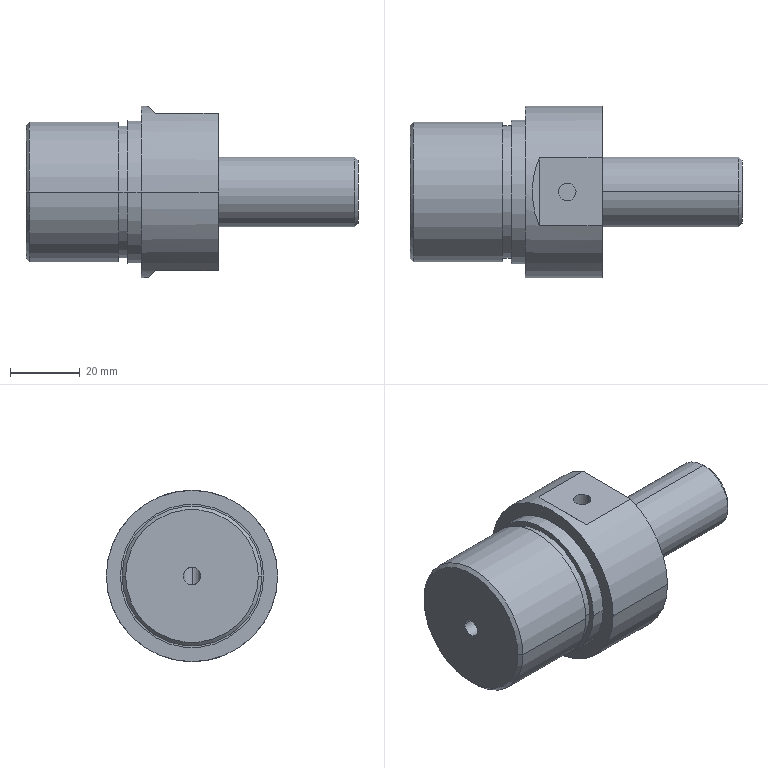Part | SolidWorks | features ICE 4, Chamfer 2, BaseBody 1, MoveFace 1 | 1 solid | 29 faces | box 95 x 49 x 49 mm | volume 93064 mm3 | cylinder 14 | plane 11 | cone 4 | commonest cylinder face diameters 5 x4 20 x2 38 x2 40 x2 41 x2 49 x2
STEP:
#1=CARTESIAN_POINT('',(82.,0.,-9.));
#2=VERTEX_POINT('',#1);
#3=CARTESIAN_POINT('',(82.,0.,9.));
#4=VERTEX_POINT('',#3);
#5=CARTESIAN_POINT('',(82.,0.,0.));
#6=DIRECTION('',(1.,0.,0.));
#7=DIRECTION('',(0.,0.,-1.));
#8=AXIS2_PLACEMENT_3D('',#5,#6,#7);
#9=CIRCLE('',#8,9.);
#10=EDGE_CURVE('',#2,#4,#9,.T.);
#11=ORIENTED_EDGE('',*,*,#10,.F.);
#12=CARTESIAN_POINT('',(81.,0.,-10.));
#13=VERTEX_POINT('',#12);
#14=CARTESIAN_POINT('',(81.,0.,-10.));
#15=DIRECTION('',(-0.7071,0.,-0.7071));
#16=VECTOR('',#15,1000.);
#17=LINE('',#14,#16);
#18=EDGE_CURVE('',#2,#13,#17,.T.);
#19=ORIENTED_EDGE('',*,*,#18,.T.);
#20=CARTESIAN_POINT('',(81.,0.,10.));
#21=VERTEX_POINT('',#20);
#22=CARTESIAN_POINT('',(81.,0.,0.));
#23=DIRECTION('',(-1.,0.,0.));
#24=DIRECTION('',(0.,0.,-1.));
#25=AXIS2_PLACEMENT_3D('',#22,#23,#24);
#26=CIRCLE('',#25,10.);
#27=EDGE_CURVE('',#21,#13,#26,.T.);
#28=ORIENTED_EDGE('',*,*,#27,.F.);
#29=CARTESIAN_POINT('',(81.,0.,10.));
#30=DIRECTION('',(-0.7071,0.,0.7071));
#31=VECTOR('',#30,1000.);
#32=LINE('',#29,#31);
#33=EDGE_CURVE('',#4,#21,#32,.T.);
#34=ORIENTED_EDGE('',*,*,#33,.F.);
#35=EDGE_LOOP('',(#11,#19,#28,#34));
#36=FACE_OUTER_BOUND('',#35,.T.);
#37=CARTESIAN_POINT('',(81.,0.,0.));
#38=DIRECTION('',(-1.,0.,0.));
#39=DIRECTION('',(0.,0.,1.));
#40=AXIS2_PLACEMENT_3D('',#37,#38,#39);
#41=CONICAL_SURFACE('',#40,10.,0.7854);
#42=ADVANCED_FACE('',(#36),#41,.T.);
#43=CARTESIAN_POINT('',(29.5,0.,-2.5));
#44=VERTEX_POINT('',#43);
#45=CARTESIAN_POINT('',(32.,2.5,0.));
#46=VERTEX_POINT('',#45);
#47=CARTESIAN_POINT('',(29.5,0.,-2.5));
#48=CARTESIAN_POINT('',(29.5,1.464,-2.5));
#49=CARTESIAN_POINT('',(30.536,2.5,-1.464));
#50=CARTESIAN_POINT('',(32.,2.5,0.));
#51=(BOUNDED_CURVE()B_SPLINE_CURVE(3,(#47,#48,#49,#50),.UNSPECIFIED.,.F.,.T.)B_SPLINE_CURVE_WITH_KNOTS((4,4),(0.,1.571),.UNSPECIFIED.)CURVE()GEOMETRIC_REPRESENTATION_ITEM()RATIONAL_B_SPLINE_CURVE((1.,0.8047,0.8047,1.))REPRESENTATION_ITEM(''));
#52=EDGE_CURVE('',#44,#46,#51,.T.);
#53=ORIENTED_EDGE('',*,*,#52,.T.);
#54=CARTESIAN_POINT('',(-13.,2.5,0.));
#55=VERTEX_POINT('',#54);
#56=CARTESIAN_POINT('',(92.001,2.5,0.));
#57=DIRECTION('',(-1.,0.,0.));
#58=VECTOR('',#57,1000.);
#59=LINE('',#56,#58);
#60=EDGE_CURVE('',#46,#55,#59,.T.);
#61=ORIENTED_EDGE('',*,*,#60,.T.);
#62=CARTESIAN_POINT('',(-13.,-2.5,0.));
#63=VERTEX_POINT('',#62);
#64=CARTESIAN_POINT('',(-13.,0.,0.));
#65=DIRECTION('',(-1.,0.,0.));
#66=DIRECTION('',(0.,-1.,0.));
#67=AXIS2_PLACEMENT_3D('',#64,#65,#66);
#68=CIRCLE('',#67,2.5);
#69=EDGE_CURVE('',#55,#63,#68,.T.);
#70=ORIENTED_EDGE('',*,*,#69,.T.);
#71=CARTESIAN_POINT('',(32.,-2.5,0.));
#72=VERTEX_POINT('',#71);
#73=CARTESIAN_POINT('',(92.001,-2.5,0.));
#74=DIRECTION('',(-1.,0.,0.));
#75=VECTOR('',#74,1000.);
#76=LINE('',#73,#75);
#77=EDGE_CURVE('',#72,#63,#76,.T.);
#78=ORIENTED_EDGE('',*,*,#77,.F.);
#79=CARTESIAN_POINT('',(32.,-2.5,0.));
#80=CARTESIAN_POINT('',(30.536,-2.5,-1.464));
#81=CARTESIAN_POINT('',(29.5,-1.464,-2.5));
#82=CARTESIAN_POINT('',(29.5,0.,-2.5));
#83=(BOUNDED_CURVE()B_SPLINE_CURVE(3,(#79,#80,#81,#82),.UNSPECIFIED.,.F.,.F.)B_SPLINE_CURVE_WITH_KNOTS((4,4),(4.712,6.283),.UNSPECIFIED.)CURVE()GEOMETRIC_REPRESENTATION_ITEM()RATIONAL_B_SPLINE_CURVE((1.,0.8047,0.8047,1.))REPRESENTATION_ITEM(''));
#84=EDGE_CURVE('',#72,#44,#83,.T.);
#85=ORIENTED_EDGE('',*,*,#84,.T.);
#86=EDGE_LOOP('',(#53,#61,#70,#78,#85));
#87=FACE_OUTER_BOUND('',#86,.T.);
#88=CARTESIAN_POINT('',(92.001,0.,0.));
#89=DIRECTION('',(-1.,0.,0.));
#90=DIRECTION('',(0.,-1.,0.));
#91=AXIS2_PLACEMENT_3D('',#88,#89,#90);
#92=CYLINDRICAL_SURFACE('',#91,2.5);
#93=ADVANCED_FACE('',(#87),#92,.F.);
#94=CARTESIAN_POINT('',(29.5,0.,2.5));
#95=VERTEX_POINT('',#94);
#96=CARTESIAN_POINT('',(29.5,0.,2.5));
#97=CARTESIAN_POINT('',(29.5,-1.464,2.5));
#98=CARTESIAN_POINT('',(30.536,-2.5,1.464));
#99=CARTESIAN_POINT('',(32.,-2.5,0.));
#100=(BOUNDED_CURVE()B_SPLINE_CURVE(3,(#96,#97,#98,#99),.UNSPECIFIED.,.F.,.T.)B_SPLINE_CURVE_WITH_KNOTS((4,4),(0.,1.571),.UNSPECIFIED.)CURVE()GEOMETRIC_REPRESENTATION_ITEM()RATIONAL_B_SPLINE_CURVE((1.,0.8047,0.8047,1.))REPRESENTATION_ITEM(''));
#101=EDGE_CURVE('',#95,#72,#100,.T.);
#102=ORIENTED_EDGE('',*,*,#101,.F.);
#103=CARTESIAN_POINT('',(29.5,0.,22.5));
#104=VERTEX_POINT('',#103);
#105=CARTESIAN_POINT('',(29.5,0.,-2.5));
#106=DIRECTION('',(0.,0.,1.));
#107=VECTOR('',#106,1000.);
#108=LINE('',#105,#107);
#109=EDGE_CURVE('',#95,#104,#108,.T.);
#110=ORIENTED_EDGE('',*,*,#109,.T.);
#111=CARTESIAN_POINT('',(34.5,0.,22.5));
#112=VERTEX_POINT('',#111);
#113=CARTESIAN_POINT('',(32.,0.,22.5));
#114=DIRECTION('',(0.,0.,1.));
#115=DIRECTION('',(1.,0.,0.));
#116=AXIS2_PLACEMENT_3D('',#113,#114,#115);
#117=CIRCLE('',#116,2.5);
#118=EDGE_CURVE('',#104,#112,#117,.T.);
#119=ORIENTED_EDGE('',*,*,#118,.T.);
#120=CARTESIAN_POINT('',(34.5,0.,-2.5));
#121=VERTEX_POINT('',#120);
#122=CARTESIAN_POINT('',(34.5,0.,-2.5));
#123=DIRECTION('',(0.,0.,1.));
#124=VECTOR('',#123,1000.);
#125=LINE('',#122,#124);
#126=EDGE_CURVE('',#121,#112,#125,.T.);
#127=ORIENTED_EDGE('',*,*,#126,.F.);
#128=CARTESIAN_POINT('',(32.,0.,-2.5));
#129=DIRECTION('',(0.,0.,1.));
#130=DIRECTION('',(1.,0.,0.));
#131=AXIS2_PLACEMENT_3D('',#128,#129,#130);
#132=CIRCLE('',#131,2.5);
#133=EDGE_CURVE('',#44,#121,#132,.T.);
#134=ORIENTED_EDGE('',*,*,#133,.F.);
#135=ORIENTED_EDGE('',*,*,#84,.F.);
#136=EDGE_LOOP('',(#102,#110,#119,#127,#134,#135));
#137=FACE_OUTER_BOUND('',#136,.T.);
#138=CARTESIAN_POINT('',(32.,0.,-2.5));
#139=DIRECTION('',(0.,0.,1.));
#140=DIRECTION('',(1.,0.,0.));
#141=AXIS2_PLACEMENT_3D('',#138,#139,#140);
#142=CYLINDRICAL_SURFACE('',#141,2.5);
#143=ADVANCED_FACE('',(#137),#142,.F.);
#144=CARTESIAN_POINT('',(42.,24.5,0.));
#145=VERTEX_POINT('',#144);
#146=CARTESIAN_POINT('',(42.,9.695,22.5));
#147=VERTEX_POINT('',#146);
#148=CARTESIAN_POINT('',(42.,0.,0.));
#149=DIRECTION('',(1.,0.,0.));
#150=DIRECTION('',(0.,-1.,0.));
#151=AXIS2_PLACEMENT_3D('',#148,#149,#150);
#152=CIRCLE('',#151,24.5);
#153=EDGE_CURVE('',#145,#147,#152,.T.);
#154=ORIENTED_EDGE('',*,*,#153,.F.);
#155=CARTESIAN_POINT('',(20.,24.5,0.));
#156=VERTEX_POINT('',#155);
#157=CARTESIAN_POINT('',(42.,24.5,0.));
#158=DIRECTION('',(-1.,0.,0.));
#159=VECTOR('',#158,1000.);
#160=LINE('',#157,#159);
#161=EDGE_CURVE('',#145,#156,#160,.T.);
#162=ORIENTED_EDGE('',*,*,#161,.T.);
#163=CARTESIAN_POINT('',(20.,-24.5,0.));
#164=VERTEX_POINT('',#163);
#165=CARTESIAN_POINT('',(20.,0.,0.));
#166=DIRECTION('',(1.,0.,0.));
#167=DIRECTION('',(0.,-1.,0.));
#168=AXIS2_PLACEMENT_3D('',#165,#166,#167);
#169=CIRCLE('',#168,24.5);
#170=EDGE_CURVE('',#156,#164,#169,.T.);
#171=ORIENTED_EDGE('',*,*,#170,.T.);
#172=CARTESIAN_POINT('',(42.,-24.5,0.));
#173=VERTEX_POINT('',#172);
#174=CARTESIAN_POINT('',(42.,-24.5,0.));
#175=DIRECTION('',(-1.,0.,0.));
#176=VECTOR('',#175,1000.);
#177=LINE('',#174,#176);
#178=EDGE_CURVE('',#173,#164,#177,.T.);
#179=ORIENTED_EDGE('',*,*,#178,.F.);
#180=CARTESIAN_POINT('',(42.,-9.695,22.5));
#181=VERTEX_POINT('',#180);
#182=CARTESIAN_POINT('',(42.,0.,0.));
#183=DIRECTION('',(1.,0.,0.));
#184=DIRECTION('',(0.,-1.,0.));
#185=AXIS2_PLACEMENT_3D('',#182,#183,#184);
#186=CIRCLE('',#185,24.5);
#187=EDGE_CURVE('',#181,#173,#186,.T.);
#188=ORIENTED_EDGE('',*,*,#187,.F.);
#189=CARTESIAN_POINT('',(24.,-9.695,22.5));
#190=VERTEX_POINT('',#189);
#191=CARTESIAN_POINT('',(42.,-9.695,22.5));
#192=DIRECTION('',(-1.,0.,0.));
#193=VECTOR('',#192,1000.);
#194=LINE('',#191,#193);
#195=EDGE_CURVE('',#181,#190,#194,.T.);
#196=ORIENTED_EDGE('',*,*,#195,.T.);
#197=CARTESIAN_POINT('',(24.,9.695,22.5));
#198=VERTEX_POINT('',#197);
#199=CARTESIAN_POINT('',(24.,-9.695,22.5));
#200=CARTESIAN_POINT('',(21.295,-3.418,25.205));
#201=CARTESIAN_POINT('',(21.295,3.418,25.205));
#202=CARTESIAN_POINT('',(24.,9.695,22.5));
#203=(BOUNDED_CURVE()B_SPLINE_CURVE(3,(#199,#200,#201,#202),.UNSPECIFIED.,.F.,.F.)B_SPLINE_CURVE_WITH_KNOTS((4,4),(5.876,6.69),.UNSPECIFIED.)CURVE()GEOMETRIC_REPRESENTATION_ITEM()RATIONAL_B_SPLINE_CURVE((1.,0.9456,0.9456,1.))REPRESENTATION_ITEM(''));
#204=EDGE_CURVE('',#190,#198,#203,.T.);
#205=ORIENTED_EDGE('',*,*,#204,.T.);
#206=CARTESIAN_POINT('',(42.,9.695,22.5));
#207=DIRECTION('',(1.,0.,0.));
#208=VECTOR('',#207,1000.);
#209=LINE('',#206,#208);
#210=EDGE_CURVE('',#198,#147,#209,.T.);
#211=ORIENTED_EDGE('',*,*,#210,.T.);
#212=EDGE_LOOP('',(#154,#162,#171,#179,#188,#196,#205,#211));
#213=FACE_OUTER_BOUND('',#212,.T.);
#214=CARTESIAN_POINT('',(42.,0.,0.));
#215=DIRECTION('',(-1.,0.,0.));
#216=DIRECTION('',(0.,-1.,0.));
#217=AXIS2_PLACEMENT_3D('',#214,#215,#216);
#218=CYLINDRICAL_SURFACE('',#217,24.5);
#219=ADVANCED_FACE('',(#213),#218,.T.);
#220=CARTESIAN_POINT('',(16.,20.5,0.));
#221=VERTEX_POINT('',#220);
#222=CARTESIAN_POINT('',(16.,-20.5,0.));
#223=VERTEX_POINT('',#222);
#224=CARTESIAN_POINT('',(16.,0.,0.));
#225=DIRECTION('',(1.,0.,0.));
#226=DIRECTION('',(0.,1.,0.));
#227=AXIS2_PLACEMENT_3D('',#224,#225,#226);
#228=CIRCLE('',#227,20.5);
#229=EDGE_CURVE('',#221,#223,#228,.T.);
#230=ORIENTED_EDGE('',*,*,#229,.T.);
#231=CARTESIAN_POINT('',(20.,-20.5,0.));
#232=VERTEX_POINT('',#231);
#233=CARTESIAN_POINT('',(16.,-20.5,0.));
#234=DIRECTION('',(1.,0.,0.));
#235=VECTOR('',#234,1000.);
#236=LINE('',#233,#235);
#237=EDGE_CURVE('',#223,#232,#236,.T.);
#238=ORIENTED_EDGE('',*,*,#237,.T.);
#239=CARTESIAN_POINT('',(20.,20.5,0.));
#240=VERTEX_POINT('',#239);
#241=CARTESIAN_POINT('',(20.,0.,0.));
#242=DIRECTION('',(1.,0.,0.));
#243=DIRECTION('',(0.,1.,0.));
#244=AXIS2_PLACEMENT_3D('',#241,#242,#243);
#245=CIRCLE('',#244,20.5);
#246=EDGE_CURVE('',#240,#232,#245,.T.);
#247=ORIENTED_EDGE('',*,*,#246,.F.);
#248=CARTESIAN_POINT('',(16.,20.5,0.));
#249=DIRECTION('',(1.,0.,0.));
#250=VECTOR('',#249,1000.);
#251=LINE('',#248,#250);
#252=EDGE_CURVE('',#221,#240,#251,.T.);
#253=ORIENTED_EDGE('',*,*,#252,.F.);
#254=EDGE_LOOP('',(#230,#238,#247,#253));
#255=FACE_OUTER_BOUND('',#254,.T.);
#256=CARTESIAN_POINT('',(16.,0.,0.));
#257=DIRECTION('',(1.,0.,0.));
#258=DIRECTION('',(0.,1.,0.));
#259=AXIS2_PLACEMENT_3D('',#256,#257,#258);
#260=CYLINDRICAL_SURFACE('',#259,20.5);
#261=ADVANCED_FACE('',(#255),#260,.T.);
#262=CARTESIAN_POINT('',(13.5,19.,0.));
#263=VERTEX_POINT('',#262);
#264=CARTESIAN_POINT('',(13.5,-19.,0.));
#265=VERTEX_POINT('',#264);
#266=CARTESIAN_POINT('',(13.5,0.,0.));
#267=DIRECTION('',(1.,0.,0.));
#268=DIRECTION('',(0.,1.,0.));
#269=AXIS2_PLACEMENT_3D('',#266,#267,#268);
#270=CIRCLE('',#269,19.);
#271=EDGE_CURVE('',#263,#265,#270,.T.);
#272=ORIENTED_EDGE('',*,*,#271,.T.);
#273=CARTESIAN_POINT('',(16.,-19.,0.));
#274=VERTEX_POINT('',#273);
#275=CARTESIAN_POINT('',(13.5,-19.,0.));
#276=DIRECTION('',(1.,0.,0.));
#277=VECTOR('',#276,1000.);
#278=LINE('',#275,#277);
#279=EDGE_CURVE('',#265,#274,#278,.T.);
#280=ORIENTED_EDGE('',*,*,#279,.T.);
#281=CARTESIAN_POINT('',(16.,19.,0.));
#282=VERTEX_POINT('',#281);
#283=CARTESIAN_POINT('',(16.,0.,0.));
#284=DIRECTION('',(1.,0.,0.));
#285=DIRECTION('',(0.,1.,0.));
#286=AXIS2_PLACEMENT_3D('',#283,#284,#285);
#287=CIRCLE('',#286,19.);
#288=EDGE_CURVE('',#282,#274,#287,.T.);
#289=ORIENTED_EDGE('',*,*,#288,.F.);
#290=CARTESIAN_POINT('',(13.5,19.,0.));
#291=DIRECTION('',(1.,0.,0.));
#292=VECTOR('',#291,1000.);
#293=LINE('',#290,#292);
#294=EDGE_CURVE('',#263,#282,#293,.T.);
#295=ORIENTED_EDGE('',*,*,#294,.F.);
#296=EDGE_LOOP('',(#272,#280,#289,#295));
#297=FACE_OUTER_BOUND('',#296,.T.);
#298=CARTESIAN_POINT('',(13.5,0.,0.));
#299=DIRECTION('',(1.,0.,0.));
#300=DIRECTION('',(0.,1.,0.));
#301=AXIS2_PLACEMENT_3D('',#298,#299,#300);
#302=CYLINDRICAL_SURFACE('',#301,19.);
#303=ADVANCED_FACE('',(#297),#302,.T.);
#304=CARTESIAN_POINT('',(-12.,20.,0.));
#305=VERTEX_POINT('',#304);
#306=CARTESIAN_POINT('',(-12.,-20.,0.));
#307=VERTEX_POINT('',#306);
#308=CARTESIAN_POINT('',(-12.,0.,0.));
#309=DIRECTION('',(1.,0.,0.));
#310=DIRECTION('',(0.,1.,0.));
#311=AXIS2_PLACEMENT_3D('',#308,#309,#310);
#312=CIRCLE('',#311,20.);
#313=EDGE_CURVE('',#305,#307,#312,.T.);
#314=ORIENTED_EDGE('',*,*,#313,.T.);
#315=CARTESIAN_POINT('',(13.5,-20.,0.));
#316=VERTEX_POINT('',#315);
#317=CARTESIAN_POINT('',(9.5,-20.,0.));
#318=DIRECTION('',(1.,0.,0.));
#319=VECTOR('',#318,1000.);
#320=LINE('',#317,#319);
#321=EDGE_CURVE('',#307,#316,#320,.T.);
#322=ORIENTED_EDGE('',*,*,#321,.T.);
#323=CARTESIAN_POINT('',(13.5,20.,0.));
#324=VERTEX_POINT('',#323);
#325=CARTESIAN_POINT('',(13.5,0.,0.));
#326=DIRECTION('',(-1.,0.,0.));
#327=DIRECTION('',(0.,1.,0.));
#328=AXIS2_PLACEMENT_3D('',#325,#326,#327);
#329=CIRCLE('',#328,20.);
#330=EDGE_CURVE('',#316,#324,#329,.T.);
#331=ORIENTED_EDGE('',*,*,#330,.T.);
#332=CARTESIAN_POINT('',(9.5,20.,0.));
#333=DIRECTION('',(1.,0.,0.));
#334=VECTOR('',#333,1000.);
#335=LINE('',#332,#334);
#336=EDGE_CURVE('',#305,#324,#335,.T.);
#337=ORIENTED_EDGE('',*,*,#336,.F.);
#338=EDGE_LOOP('',(#314,#322,#331,#337));
#339=FACE_OUTER_BOUND('',#338,.T.);
#340=CARTESIAN_POINT('',(9.5,0.,0.));
#341=DIRECTION('',(1.,0.,0.));
#342=DIRECTION('',(0.,1.,0.));
#343=AXIS2_PLACEMENT_3D('',#340,#341,#342);
#344=CYLINDRICAL_SURFACE('',#343,20.);
#345=ADVANCED_FACE('',(#339),#344,.T.);
#346=CARTESIAN_POINT('',(-13.,19.,0.));
#347=VERTEX_POINT('',#346);
#348=CARTESIAN_POINT('',(-13.,-19.,0.));
#349=VERTEX_POINT('',#348);
#350=CARTESIAN_POINT('',(-13.,0.,0.));
#351=DIRECTION('',(1.,0.,0.));
#352=DIRECTION('',(0.,1.,0.));
#353=AXIS2_PLACEMENT_3D('',#350,#351,#352);
#354=CIRCLE('',#353,19.);
#355=EDGE_CURVE('',#347,#349,#354,.T.);
#356=ORIENTED_EDGE('',*,*,#355,.T.);
#357=CARTESIAN_POINT('',(-12.,-20.,0.));
#358=DIRECTION('',(0.7071,-0.7071,0.));
#359=VECTOR('',#358,1000.);
#360=LINE('',#357,#359);
#361=EDGE_CURVE('',#349,#307,#360,.T.);
#362=ORIENTED_EDGE('',*,*,#361,.T.);
#363=ORIENTED_EDGE('',*,*,#313,.F.);
#364=CARTESIAN_POINT('',(-12.,20.,0.));
#365=DIRECTION('',(0.7071,0.7071,0.));
#366=VECTOR('',#365,1000.);
#367=LINE('',#364,#366);
#368=EDGE_CURVE('',#347,#305,#367,.T.);
#369=ORIENTED_EDGE('',*,*,#368,.F.);
#370=EDGE_LOOP('',(#356,#362,#363,#369));
#371=FACE_OUTER_BOUND('',#370,.T.);
#372=CARTESIAN_POINT('',(-12.,0.,0.));
#373=DIRECTION('',(1.,0.,0.));
#374=DIRECTION('',(0.,1.,0.));
#375=AXIS2_PLACEMENT_3D('',#372,#373,#374);
#376=CONICAL_SURFACE('',#375,20.,0.7854);
#377=ADVANCED_FACE('',(#371),#376,.T.);
#378=CARTESIAN_POINT('',(42.,0.,10.));
#379=VERTEX_POINT('',#378);
#380=CARTESIAN_POINT('',(42.,0.,-10.));
#381=VERTEX_POINT('',#380);
#382=CARTESIAN_POINT('',(42.,0.,0.));
#383=DIRECTION('',(-1.,0.,0.));
#384=DIRECTION('',(0.,0.,-1.));
#385=AXIS2_PLACEMENT_3D('',#382,#383,#384);
#386=CIRCLE('',#385,10.);
#387=EDGE_CURVE('',#379,#381,#386,.T.);
#388=ORIENTED_EDGE('',*,*,#387,.F.);
#389=CARTESIAN_POINT('',(-17.98,0.,10.));
#390=DIRECTION('',(1.,0.,0.));
#391=VECTOR('',#390,1000.);
#392=LINE('',#389,#391);
#393=EDGE_CURVE('',#379,#21,#392,.T.);
#394=ORIENTED_EDGE('',*,*,#393,.T.);
#395=ORIENTED_EDGE('',*,*,#27,.T.);
#396=CARTESIAN_POINT('',(-17.98,0.,-10.));
#397=DIRECTION('',(1.,0.,0.));
#398=VECTOR('',#397,1000.);
#399=LINE('',#396,#398);
#400=EDGE_CURVE('',#381,#13,#399,.T.);
#401=ORIENTED_EDGE('',*,*,#400,.F.);
#402=EDGE_LOOP('',(#388,#394,#395,#401));
#403=FACE_OUTER_BOUND('',#402,.T.);
#404=CARTESIAN_POINT('',(-17.98,0.,0.));
#405=DIRECTION('',(1.,0.,0.));
#406=DIRECTION('',(0.,0.,-1.));
#407=AXIS2_PLACEMENT_3D('',#404,#405,#406);
#408=CYLINDRICAL_SURFACE('',#407,10.);
#409=ADVANCED_FACE('',(#403),#408,.T.);
#410=ORIENTED_EDGE('',*,*,#393,.F.);
#411=CARTESIAN_POINT('',(42.,0.,0.));
#412=DIRECTION('',(-1.,0.,0.));
#413=DIRECTION('',(0.,0.,-1.));
#414=AXIS2_PLACEMENT_3D('',#411,#412,#413);
#415=CIRCLE('',#414,10.);
#416=EDGE_CURVE('',#381,#379,#415,.T.);
#417=ORIENTED_EDGE('',*,*,#416,.F.);
#418=ORIENTED_EDGE('',*,*,#400,.T.);
#419=CARTESIAN_POINT('',(81.,0.,0.));
#420=DIRECTION('',(-1.,0.,0.));
#421=DIRECTION('',(0.,0.,-1.));
#422=AXIS2_PLACEMENT_3D('',#419,#420,#421);
#423=CIRCLE('',#422,10.);
#424=EDGE_CURVE('',#13,#21,#423,.T.);
#425=ORIENTED_EDGE('',*,*,#424,.T.);
#426=EDGE_LOOP('',(#410,#417,#418,#425));
#427=FACE_OUTER_BOUND('',#426,.T.);
#428=CARTESIAN_POINT('',(-17.98,0.,0.));
#429=DIRECTION('',(1.,0.,0.));
#430=DIRECTION('',(0.,0.,-1.));
#431=AXIS2_PLACEMENT_3D('',#428,#429,#430);
#432=CYLINDRICAL_SURFACE('',#431,10.);
#433=ADVANCED_FACE('',(#427),#432,.T.);
#434=CARTESIAN_POINT('',(42.,21.5,22.5));
#435=DIRECTION('',(0.,-1.,0.));
#436=VECTOR('',#435,1000.);
#437=LINE('',#434,#436);
#438=EDGE_CURVE('',#147,#181,#437,.T.);
#439=ORIENTED_EDGE('',*,*,#438,.T.);
#440=ORIENTED_EDGE('',*,*,#187,.T.);
#441=CARTESIAN_POINT('',(42.,-9.695,-22.5));
#442=VERTEX_POINT('',#441);
#443=CARTESIAN_POINT('',(42.,0.,0.));
#444=DIRECTION('',(1.,0.,0.));
#445=DIRECTION('',(0.,-1.,0.));
#446=AXIS2_PLACEMENT_3D('',#443,#444,#445);
#447=CIRCLE('',#446,24.5);
#448=EDGE_CURVE('',#173,#442,#447,.T.);
#449=ORIENTED_EDGE('',*,*,#448,.T.);
#450=CARTESIAN_POINT('',(42.,9.695,-22.5));
#451=VERTEX_POINT('',#450);
#452=CARTESIAN_POINT('',(42.,21.5,-22.5));
#453=DIRECTION('',(0.,1.,0.));
#454=VECTOR('',#453,1000.);
#455=LINE('',#452,#454);
#456=EDGE_CURVE('',#442,#451,#455,.T.);
#457=ORIENTED_EDGE('',*,*,#456,.T.);
#458=CARTESIAN_POINT('',(42.,0.,0.));
#459=DIRECTION('',(1.,0.,0.));
#460=DIRECTION('',(0.,-1.,0.));
#461=AXIS2_PLACEMENT_3D('',#458,#459,#460);
#462=CIRCLE('',#461,24.5);
#463=EDGE_CURVE('',#451,#145,#462,.T.);
#464=ORIENTED_EDGE('',*,*,#463,.T.);
#465=ORIENTED_EDGE('',*,*,#153,.T.);
#466=EDGE_LOOP('',(#439,#440,#449,#457,#464,#465));
#467=FACE_OUTER_BOUND('',#466,.T.);
#468=ORIENTED_EDGE('',*,*,#416,.T.);
#469=ORIENTED_EDGE('',*,*,#387,.T.);
#470=EDGE_LOOP('',(#468,#469));
#471=FACE_BOUND('',#470,.T.);
#472=CARTESIAN_POINT('',(42.,21.5,0.));
#473=DIRECTION('',(1.,0.,0.));
#474=DIRECTION('',(0.,0.,-1.));
#475=AXIS2_PLACEMENT_3D('',#472,#473,#474);
#476=PLANE('',#475);
#477=ADVANCED_FACE('',(#467,#471),#476,.T.);
#478=ORIENTED_EDGE('',*,*,#161,.F.);
#479=ORIENTED_EDGE('',*,*,#463,.F.);
#480=CARTESIAN_POINT('',(24.,9.695,-22.5));
#481=VERTEX_POINT('',#480);
#482=CARTESIAN_POINT('',(42.,9.695,-22.5));
#483=DIRECTION('',(-1.,0.,0.));
#484=VECTOR('',#483,1000.);
#485=LINE('',#482,#484);
#486=EDGE_CURVE('',#451,#481,#485,.T.);
#487=ORIENTED_EDGE('',*,*,#486,.T.);
#488=CARTESIAN_POINT('',(24.,-9.695,-22.5));
#489=VERTEX_POINT('',#488);
#490=CARTESIAN_POINT('',(24.,9.695,-22.5));
#491=CARTESIAN_POINT('',(21.295,3.418,-25.205));
#492=CARTESIAN_POINT('',(21.295,-3.418,-25.205));
#493=CARTESIAN_POINT('',(24.,-9.695,-22.5));
#494=(BOUNDED_CURVE()B_SPLINE_CURVE(3,(#490,#491,#492,#493),.UNSPECIFIED.,.F.,.F.)B_SPLINE_CURVE_WITH_KNOTS((4,4),(5.876,6.69),.UNSPECIFIED.)CURVE()GEOMETRIC_REPRESENTATION_ITEM()RATIONAL_B_SPLINE_CURVE((1.,0.9456,0.9456,1.))REPRESENTATION_ITEM(''));
#495=EDGE_CURVE('',#481,#489,#494,.T.);
#496=ORIENTED_EDGE('',*,*,#495,.T.);
#497=CARTESIAN_POINT('',(42.,-9.695,-22.5));
#498=DIRECTION('',(1.,0.,0.));
#499=VECTOR('',#498,1000.);
#500=LINE('',#497,#499);
#501=EDGE_CURVE('',#489,#442,#500,.T.);
#502=ORIENTED_EDGE('',*,*,#501,.T.);
#503=ORIENTED_EDGE('',*,*,#448,.F.);
#504=ORIENTED_EDGE('',*,*,#178,.T.);
#505=CARTESIAN_POINT('',(20.,0.,0.));
#506=DIRECTION('',(1.,0.,0.));
#507=DIRECTION('',(0.,-1.,0.));
#508=AXIS2_PLACEMENT_3D('',#505,#506,#507);
#509=CIRCLE('',#508,24.5);
#510=EDGE_CURVE('',#164,#156,#509,.T.);
#511=ORIENTED_EDGE('',*,*,#510,.T.);
#512=EDGE_LOOP('',(#478,#479,#487,#496,#502,#503,#504,#511));
#513=FACE_OUTER_BOUND('',#512,.T.);
#514=CARTESIAN_POINT('',(42.,0.,0.));
#515=DIRECTION('',(-1.,0.,0.));
#516=DIRECTION('',(0.,-1.,0.));
#517=AXIS2_PLACEMENT_3D('',#514,#515,#516);
#518=CYLINDRICAL_SURFACE('',#517,24.5);
#519=ADVANCED_FACE('',(#513),#518,.T.);
#520=CARTESIAN_POINT('',(32.,0.,22.5));
#521=DIRECTION('',(0.,0.,1.));
#522=DIRECTION('',(1.,0.,0.));
#523=AXIS2_PLACEMENT_3D('',#520,#521,#522);
#524=CIRCLE('',#523,2.5);
#525=EDGE_CURVE('',#112,#104,#524,.T.);
#526=ORIENTED_EDGE('',*,*,#525,.F.);
#527=ORIENTED_EDGE('',*,*,#118,.F.);
#528=EDGE_LOOP('',(#526,#527));
#529=FACE_BOUND('',#528,.T.);
#530=ORIENTED_EDGE('',*,*,#438,.F.);
#531=ORIENTED_EDGE('',*,*,#210,.F.);
#532=CARTESIAN_POINT('',(24.,0.,22.5));
#533=DIRECTION('',(0.,1.,0.));
#534=VECTOR('',#533,1000.);
#535=LINE('',#532,#534);
#536=EDGE_CURVE('',#190,#198,#535,.T.);
#537=ORIENTED_EDGE('',*,*,#536,.F.);
#538=ORIENTED_EDGE('',*,*,#195,.F.);
#539=EDGE_LOOP('',(#530,#531,#537,#538));
#540=FACE_OUTER_BOUND('',#539,.T.);
#541=CARTESIAN_POINT('',(42.,0.,22.5));
#542=DIRECTION('',(0.,0.,-1.));
#543=DIRECTION('',(-1.,0.,0.));
#544=AXIS2_PLACEMENT_3D('',#541,#542,#543);
#545=PLANE('',#544);
#546=ADVANCED_FACE('',(#529,#540),#545,.F.);
#547=ORIENTED_EDGE('',*,*,#456,.F.);
#548=ORIENTED_EDGE('',*,*,#501,.F.);
#549=CARTESIAN_POINT('',(24.,0.,-22.5));
#550=DIRECTION('',(0.,-1.,0.));
#551=VECTOR('',#550,1000.);
#552=LINE('',#549,#551);
#553=EDGE_CURVE('',#481,#489,#552,.T.);
#554=ORIENTED_EDGE('',*,*,#553,.F.);
#555=ORIENTED_EDGE('',*,*,#486,.F.);
#556=EDGE_LOOP('',(#547,#548,#554,#555));
#557=FACE_OUTER_BOUND('',#556,.T.);
#558=CARTESIAN_POINT('',(42.,0.,-22.5));
#559=DIRECTION('',(0.,0.,1.));
#560=DIRECTION('',(1.,0.,0.));
#561=AXIS2_PLACEMENT_3D('',#558,#559,#560);
#562=PLANE('',#561);
#563=ADVANCED_FACE('',(#557),#562,.F.);
#564=ORIENTED_EDGE('',*,*,#246,.T.);
#565=CARTESIAN_POINT('',(20.,0.,0.));
#566=DIRECTION('',(1.,0.,0.));
#567=DIRECTION('',(0.,1.,0.));
#568=AXIS2_PLACEMENT_3D('',#565,#566,#567);
#569=CIRCLE('',#568,20.5);
#570=EDGE_CURVE('',#232,#240,#569,.T.);
#571=ORIENTED_EDGE('',*,*,#570,.T.);
#572=EDGE_LOOP('',(#564,#571));
#573=FACE_BOUND('',#572,.T.);
#574=ORIENTED_EDGE('',*,*,#510,.F.);
#575=ORIENTED_EDGE('',*,*,#170,.F.);
#576=EDGE_LOOP('',(#574,#575));
#577=FACE_OUTER_BOUND('',#576,.T.);
#578=CARTESIAN_POINT('',(20.,22.5,0.));
#579=DIRECTION('',(-1.,0.,0.));
#580=DIRECTION('',(0.,-1.,0.));
#581=AXIS2_PLACEMENT_3D('',#578,#579,#580);
#582=PLANE('',#581);
#583=ADVANCED_FACE('',(#573,#577),#582,.T.);
#584=ORIENTED_EDGE('',*,*,#553,.T.);
#585=ORIENTED_EDGE('',*,*,#495,.F.);
#586=EDGE_LOOP('',(#584,#585));
#587=FACE_OUTER_BOUND('',#586,.T.);
#588=CARTESIAN_POINT('',(24.,0.,-22.5));
#589=DIRECTION('',(0.7071,0.,-0.7071));
#590=DIRECTION('',(-0.7071,0.,-0.7071));
#591=AXIS2_PLACEMENT_3D('',#588,#589,#590);
#592=PLANE('',#591);
#593=ADVANCED_FACE('',(#587),#592,.T.);
#594=ORIENTED_EDGE('',*,*,#536,.T.);
#595=ORIENTED_EDGE('',*,*,#204,.F.);
#596=EDGE_LOOP('',(#594,#595));
#597=FACE_OUTER_BOUND('',#596,.T.);
#598=CARTESIAN_POINT('',(24.,0.,22.5));
#599=DIRECTION('',(0.7071,0.,0.7071));
#600=DIRECTION('',(0.7071,0.,-0.7071));
#601=AXIS2_PLACEMENT_3D('',#598,#599,#600);
#602=PLANE('',#601);
#603=ADVANCED_FACE('',(#597),#602,.T.);
#604=ORIENTED_EDGE('',*,*,#237,.F.);
#605=CARTESIAN_POINT('',(16.,0.,0.));
#606=DIRECTION('',(1.,0.,0.));
#607=DIRECTION('',(0.,1.,0.));
#608=AXIS2_PLACEMENT_3D('',#605,#606,#607);
#609=CIRCLE('',#608,20.5);
#610=EDGE_CURVE('',#223,#221,#609,.T.);
#611=ORIENTED_EDGE('',*,*,#610,.T.);
#612=ORIENTED_EDGE('',*,*,#252,.T.);
#613=ORIENTED_EDGE('',*,*,#570,.F.);
#614=EDGE_LOOP('',(#604,#611,#612,#613));
#615=FACE_OUTER_BOUND('',#614,.T.);
#616=CARTESIAN_POINT('',(16.,0.,0.));
#617=DIRECTION('',(1.,0.,0.));
#618=DIRECTION('',(0.,1.,0.));
#619=AXIS2_PLACEMENT_3D('',#616,#617,#618);
#620=CYLINDRICAL_SURFACE('',#619,20.5);
#621=ADVANCED_FACE('',(#615),#620,.T.);
#622=ORIENTED_EDGE('',*,*,#288,.T.);
#623=CARTESIAN_POINT('',(16.,0.,0.));
#624=DIRECTION('',(1.,0.,0.));
#625=DIRECTION('',(0.,1.,0.));
#626=AXIS2_PLACEMENT_3D('',#623,#624,#625);
#627=CIRCLE('',#626,19.);
#628=EDGE_CURVE('',#274,#282,#627,.T.);
#629=ORIENTED_EDGE('',*,*,#628,.T.);
#630=EDGE_LOOP('',(#622,#629));
#631=FACE_BOUND('',#630,.T.);
#632=ORIENTED_EDGE('',*,*,#229,.F.);
#633=ORIENTED_EDGE('',*,*,#610,.F.);
#634=EDGE_LOOP('',(#632,#633));
#635=FACE_OUTER_BOUND('',#634,.T.);
#636=CARTESIAN_POINT('',(16.,0.,0.));
#637=DIRECTION('',(-1.,0.,0.));
#638=DIRECTION('',(0.,-1.,0.));
#639=AXIS2_PLACEMENT_3D('',#636,#637,#638);
#640=PLANE('',#639);
#641=ADVANCED_FACE('',(#631,#635),#640,.T.);
#642=ORIENTED_EDGE('',*,*,#279,.F.);
#643=CARTESIAN_POINT('',(13.5,0.,0.));
#644=DIRECTION('',(1.,0.,0.));
#645=DIRECTION('',(0.,1.,0.));
#646=AXIS2_PLACEMENT_3D('',#643,#644,#645);
#647=CIRCLE('',#646,19.);
#648=EDGE_CURVE('',#265,#263,#647,.T.);
#649=ORIENTED_EDGE('',*,*,#648,.T.);
#650=ORIENTED_EDGE('',*,*,#294,.T.);
#651=ORIENTED_EDGE('',*,*,#628,.F.);
#652=EDGE_LOOP('',(#642,#649,#650,#651));
#653=FACE_OUTER_BOUND('',#652,.T.);
#654=CARTESIAN_POINT('',(13.5,0.,0.));
#655=DIRECTION('',(1.,0.,0.));
#656=DIRECTION('',(0.,1.,0.));
#657=AXIS2_PLACEMENT_3D('',#654,#655,#656);
#658=CYLINDRICAL_SURFACE('',#657,19.);
#659=ADVANCED_FACE('',(#653),#658,.T.);
#660=ORIENTED_EDGE('',*,*,#271,.F.);
#661=ORIENTED_EDGE('',*,*,#648,.F.);
#662=EDGE_LOOP('',(#660,#661));
#663=FACE_BOUND('',#662,.T.);
#664=CARTESIAN_POINT('',(13.5,0.,0.));
#665=DIRECTION('',(-1.,0.,0.));
#666=DIRECTION('',(0.,1.,0.));
#667=AXIS2_PLACEMENT_3D('',#664,#665,#666);
#668=CIRCLE('',#667,20.);
#669=EDGE_CURVE('',#324,#316,#668,.T.);
#670=ORIENTED_EDGE('',*,*,#669,.F.);
#671=ORIENTED_EDGE('',*,*,#330,.F.);
#672=EDGE_LOOP('',(#670,#671));
#673=FACE_OUTER_BOUND('',#672,.T.);
#674=CARTESIAN_POINT('',(13.5,0.,0.));
#675=DIRECTION('',(-1.,0.,0.));
#676=DIRECTION('',(0.,-1.,0.));
#677=AXIS2_PLACEMENT_3D('',#674,#675,#676);
#678=PLANE('',#677);
#679=ADVANCED_FACE('',(#663,#673),#678,.F.);
#680=ORIENTED_EDGE('',*,*,#321,.F.);
#681=CARTESIAN_POINT('',(-12.,0.,0.));
#682=DIRECTION('',(1.,0.,0.));
#683=DIRECTION('',(0.,1.,0.));
#684=AXIS2_PLACEMENT_3D('',#681,#682,#683);
#685=CIRCLE('',#684,20.);
#686=EDGE_CURVE('',#307,#305,#685,.T.);
#687=ORIENTED_EDGE('',*,*,#686,.T.);
#688=ORIENTED_EDGE('',*,*,#336,.T.);
#689=ORIENTED_EDGE('',*,*,#669,.T.);
#690=EDGE_LOOP('',(#680,#687,#688,#689));
#691=FACE_OUTER_BOUND('',#690,.T.);
#692=CARTESIAN_POINT('',(9.5,0.,0.));
#693=DIRECTION('',(1.,0.,0.));
#694=DIRECTION('',(0.,1.,0.));
#695=AXIS2_PLACEMENT_3D('',#692,#693,#694);
#696=CYLINDRICAL_SURFACE('',#695,20.);
#697=ADVANCED_FACE('',(#691),#696,.T.);
#698=ORIENTED_EDGE('',*,*,#361,.F.);
#699=CARTESIAN_POINT('',(-13.,0.,0.));
#700=DIRECTION('',(1.,0.,0.));
#701=DIRECTION('',(0.,1.,0.));
#702=AXIS2_PLACEMENT_3D('',#699,#700,#701);
#703=CIRCLE('',#702,19.);
#704=EDGE_CURVE('',#349,#347,#703,.T.);
#705=ORIENTED_EDGE('',*,*,#704,.T.);
#706=ORIENTED_EDGE('',*,*,#368,.T.);
#707=ORIENTED_EDGE('',*,*,#686,.F.);
#708=EDGE_LOOP('',(#698,#705,#706,#707));
#709=FACE_OUTER_BOUND('',#708,.T.);
#710=CARTESIAN_POINT('',(-12.,0.,0.));
#711=DIRECTION('',(1.,0.,0.));
#712=DIRECTION('',(0.,1.,0.));
#713=AXIS2_PLACEMENT_3D('',#710,#711,#712);
#714=CONICAL_SURFACE('',#713,20.,0.7854);
#715=ADVANCED_FACE('',(#709),#714,.T.);
#716=CARTESIAN_POINT('',(-13.,0.,0.));
#717=DIRECTION('',(-1.,0.,0.));
#718=DIRECTION('',(0.,-1.,0.));
#719=AXIS2_PLACEMENT_3D('',#716,#717,#718);
#720=CIRCLE('',#719,2.5);
#721=EDGE_CURVE('',#63,#55,#720,.T.);
#722=ORIENTED_EDGE('',*,*,#721,.F.);
#723=ORIENTED_EDGE('',*,*,#69,.F.);
#724=EDGE_LOOP('',(#722,#723));
#725=FACE_BOUND('',#724,.T.);
#726=ORIENTED_EDGE('',*,*,#355,.F.);
#727=ORIENTED_EDGE('',*,*,#704,.F.);
#728=EDGE_LOOP('',(#726,#727));
#729=FACE_OUTER_BOUND('',#728,.T.);
#730=CARTESIAN_POINT('',(-13.,0.,0.));
#731=DIRECTION('',(1.,0.,0.));
#732=DIRECTION('',(0.,1.,0.));
#733=AXIS2_PLACEMENT_3D('',#730,#731,#732);
#734=PLANE('',#733);
#735=ADVANCED_FACE('',(#725,#729),#734,.F.);
#736=ORIENTED_EDGE('',*,*,#109,.F.);
#737=CARTESIAN_POINT('',(32.,2.5,0.));
#738=CARTESIAN_POINT('',(30.536,2.5,1.464));
#739=CARTESIAN_POINT('',(29.5,1.464,2.5));
#740=CARTESIAN_POINT('',(29.5,0.,2.5));
#741=(BOUNDED_CURVE()B_SPLINE_CURVE(3,(#737,#738,#739,#740),.UNSPECIFIED.,.F.,.T.)B_SPLINE_CURVE_WITH_KNOTS((4,4),(4.712,6.283),.UNSPECIFIED.)CURVE()GEOMETRIC_REPRESENTATION_ITEM()RATIONAL_B_SPLINE_CURVE((1.,0.8047,0.8047,1.))REPRESENTATION_ITEM(''));
#742=EDGE_CURVE('',#46,#95,#741,.T.);
#743=ORIENTED_EDGE('',*,*,#742,.F.);
#744=ORIENTED_EDGE('',*,*,#52,.F.);
#745=CARTESIAN_POINT('',(32.,0.,-2.5));
#746=DIRECTION('',(0.,0.,1.));
#747=DIRECTION('',(1.,0.,0.));
#748=AXIS2_PLACEMENT_3D('',#745,#746,#747);
#749=CIRCLE('',#748,2.5);
#750=EDGE_CURVE('',#121,#44,#749,.T.);
#751=ORIENTED_EDGE('',*,*,#750,.F.);
#752=ORIENTED_EDGE('',*,*,#126,.T.);
#753=ORIENTED_EDGE('',*,*,#525,.T.);
#754=EDGE_LOOP('',(#736,#743,#744,#751,#752,#753));
#755=FACE_OUTER_BOUND('',#754,.T.);
#756=CARTESIAN_POINT('',(32.,0.,-2.5));
#757=DIRECTION('',(0.,0.,1.));
#758=DIRECTION('',(1.,0.,0.));
#759=AXIS2_PLACEMENT_3D('',#756,#757,#758);
#760=CYLINDRICAL_SURFACE('',#759,2.5);
#761=ADVANCED_FACE('',(#755),#760,.F.);
#762=ORIENTED_EDGE('',*,*,#133,.T.);
#763=ORIENTED_EDGE('',*,*,#750,.T.);
#764=EDGE_LOOP('',(#762,#763));
#765=FACE_OUTER_BOUND('',#764,.T.);
#766=CARTESIAN_POINT('',(32.,0.,-2.5));
#767=DIRECTION('',(0.,0.,1.));
#768=DIRECTION('',(1.,0.,0.));
#769=AXIS2_PLACEMENT_3D('',#766,#767,#768);
#770=PLANE('',#769);
#771=ADVANCED_FACE('',(#765),#770,.T.);
#772=ORIENTED_EDGE('',*,*,#60,.F.);
#773=ORIENTED_EDGE('',*,*,#742,.T.);
#774=ORIENTED_EDGE('',*,*,#101,.T.);
#775=ORIENTED_EDGE('',*,*,#77,.T.);
#776=ORIENTED_EDGE('',*,*,#721,.T.);
#777=EDGE_LOOP('',(#772,#773,#774,#775,#776));
#778=FACE_OUTER_BOUND('',#777,.T.);
#779=CARTESIAN_POINT('',(92.001,0.,0.));
#780=DIRECTION('',(-1.,0.,0.));
#781=DIRECTION('',(0.,-1.,0.));
#782=AXIS2_PLACEMENT_3D('',#779,#780,#781);
#783=CYLINDRICAL_SURFACE('',#782,2.5);
#784=ADVANCED_FACE('',(#778),#783,.F.);
#785=CARTESIAN_POINT('',(82.,0.,0.));
#786=DIRECTION('',(1.,0.,0.));
#787=DIRECTION('',(0.,0.,-1.));
#788=AXIS2_PLACEMENT_3D('',#785,#786,#787);
#789=CIRCLE('',#788,9.);
#790=EDGE_CURVE('',#4,#2,#789,.T.);
#791=ORIENTED_EDGE('',*,*,#790,.T.);
#792=ORIENTED_EDGE('',*,*,#10,.T.);
#793=EDGE_LOOP('',(#791,#792));
#794=FACE_OUTER_BOUND('',#793,.T.);
#795=CARTESIAN_POINT('',(82.,0.,0.));
#796=DIRECTION('',(1.,0.,0.));
#797=DIRECTION('',(0.,0.,-1.));
#798=AXIS2_PLACEMENT_3D('',#795,#796,#797);
#799=PLANE('',#798);
#800=ADVANCED_FACE('',(#794),#799,.T.);
#801=ORIENTED_EDGE('',*,*,#18,.F.);
#802=ORIENTED_EDGE('',*,*,#790,.F.);
#803=ORIENTED_EDGE('',*,*,#33,.T.);
#804=ORIENTED_EDGE('',*,*,#424,.F.);
#805=EDGE_LOOP('',(#801,#802,#803,#804));
#806=FACE_OUTER_BOUND('',#805,.T.);
#807=CARTESIAN_POINT('',(81.,0.,0.));
#808=DIRECTION('',(-1.,0.,0.));
#809=DIRECTION('',(0.,0.,1.));
#810=AXIS2_PLACEMENT_3D('',#807,#808,#809);
#811=CONICAL_SURFACE('',#810,10.,0.7854);
#812=ADVANCED_FACE('',(#806),#811,.T.);
#813=CLOSED_SHELL('',(#42,#93,#143,#219,#261,#303,#345,#377,#409,#433,#477,#519,#546,#563,#583,#593,#603,#621,#641,#659,#679,#697,#715,#735,#761,#771,#784,#800,#812));
#814=MANIFOLD_SOLID_BREP('',#813);
#815=CARTESIAN_POINT('',(0.,0.,0.));
#816=DIRECTION('',(0.,0.,1.));
#817=DIRECTION('',(1.,0.,0.));
#818=AXIS2_PLACEMENT_3D('',#815,#816,#817);
#819=(LENGTH_UNIT()NAMED_UNIT(*)SI_UNIT(.MILLI.,.METRE.));
#820=UNCERTAINTY_MEASURE_WITH_UNIT(LENGTH_MEASURE(0.00001),#819,'','');
#821=(NAMED_UNIT(*)PLANE_ANGLE_UNIT()SI_UNIT($,.RADIAN.));
#822=(NAMED_UNIT(*)SI_UNIT($,.STERADIAN.)SOLID_ANGLE_UNIT());
#823=(GEOMETRIC_REPRESENTATION_CONTEXT(3)GLOBAL_UNCERTAINTY_ASSIGNED_CONTEXT((#820))GLOBAL_UNIT_ASSIGNED_CONTEXT((#819,#821,#822))REPRESENTATION_CONTEXT('',''));
#824=ADVANCED_BREP_SHAPE_REPRESENTATION('',(#814,#818),#823);